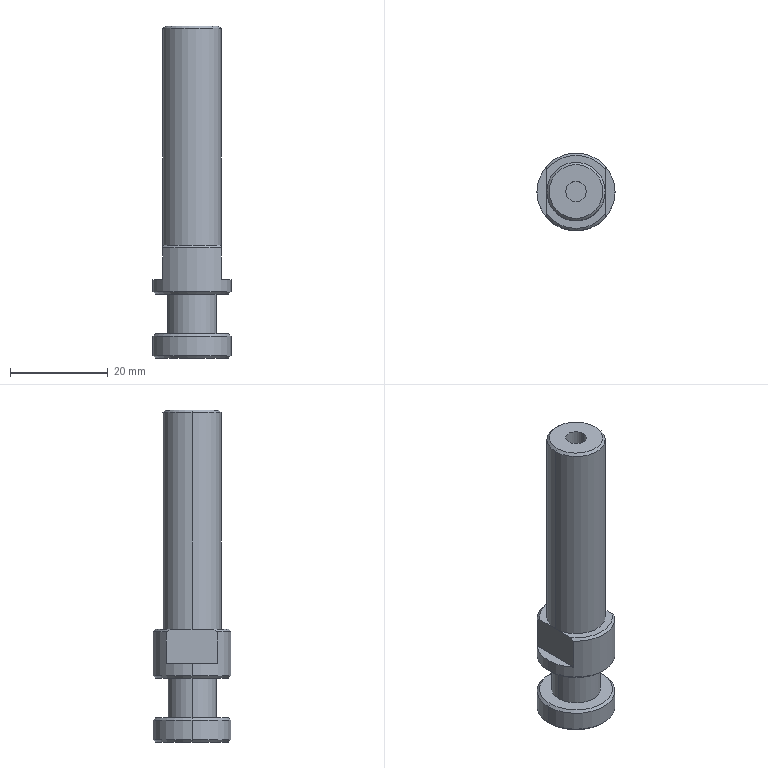Part | STEP file | PN_0068 Mount electronic clip s horizontal manipulator movable head | 1 solid | 31 faces | box 16 x 16 x 68.1 mm | volume 8318 mm3 | plane 11 | cone 10 | cylinder 10 | commonest cylinder face diameters 16 x4 4.2 x2 10 x2 12 x2